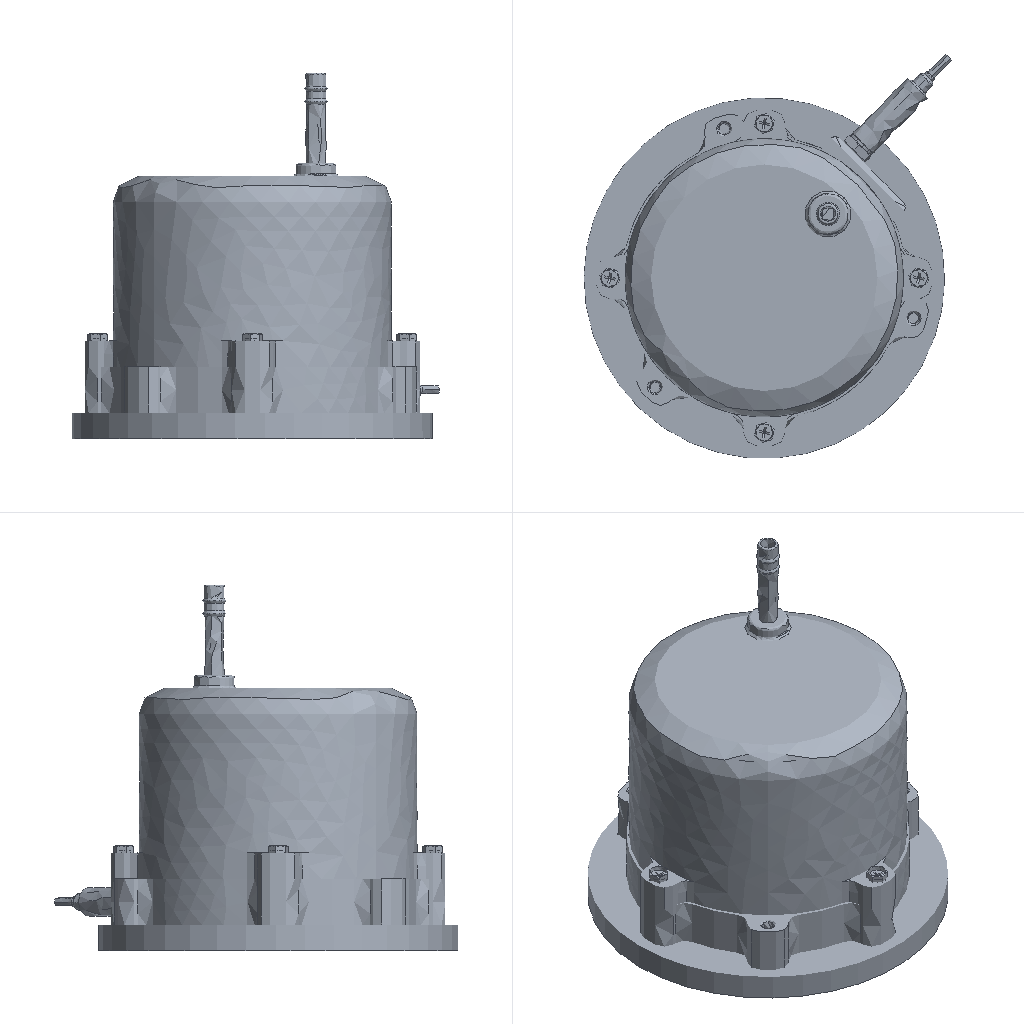Simulation study | ansys workbench
Ansys APDL input file, long lists of numbers shortened:
/batch
/config,noeldb,1     ! force off writing results to database
*get,_wallstrt,active,,time,wall
! ANSYS input file written by Workbench version 2022 R1
! File used for geometry attach:
/title,_________--__ (B5)
! ****** Begin Custom Load Command Snippet ******
/COM, ACT Extensions:
/COM,     LSDYNA, 2021.1
/COM,
! ****** End   Custom Load Command Snippet ******
*DIM,_wb_ProjectScratch_dir,string,248
_wb_ProjectScratch_dir(1) = ''
*DIM,_wb_SolverFiles_dir,string,248
_wb_SolverFiles_dir(1) = ''
*DIM,_wb_userfiles_dir,string,248
_wb_userfiles_dir(1) = ''
/com,--- Data in consistent NMM units. See Solving Units in the help system for more information.
/units,MPA
/nopr
/wb,file,start              !  signify a WB generated input file
/prep7
! Turn off shape checking because checks already performed inside WB mesher.
! See help system for more information.
SHPP,OFF,,NOWARN
/nolist
etcon,set             ! allow ANSYS to choose best KEYOP's for 180x elements, resets any applicable keyopt to MAPDL defaults
/com,*********** Nodes for the whole assembly ***********
nblock,3,,121147
(1i9,3e20.9e3)
        1    -1.317994642E+02     2.267337416E+01     2.460000000E+01
! (110133 more lines like these left out)
-1
/wb,elem,start            !  set before creation of elements
/com,*********** Elements for Body 1 "___|__-__3" ***********
et,1,187
eblock,19,solid,,437
(19i9)
        1        1        1        1        0        0        0        0       10        0     4342    11800    11908    11828    11837    12339    12480    12336    12337
! (873 more lines like these left out)
-1
/com,*********** Elements for Body 2 "__|__1" ***********
et,2,187
eblock,19,solid,,16989
(19i9)
        2        2        2        2        0        0        0        0       10        0    40629    81691    81703    85517    85507    90407    90536    90413    90412
! (33977 more lines like these left out)
-1
/com,*********** Elements for Body 3 "___|__-__1" ***********
et,3,186
keyo,3,2,1          ! set full integration on SOLID186
eblock,19,solid,,126
(19i9)
        3        3        3        3        0        0        0        0       20        0     2518     7295     7301     7355     7349     7392     7391     7382     7383
! (251 more lines like these left out)
-1
/com,*********** Elements for Body 4 "_|__-__3" ***********
et,4,187
eblock,19,solid,,3042
(19i9)
        4        4        4        4        0        0        0        0       10        0    14075    32512    32947    32813    32928    35736    37332    35733    35735
! (6083 more lines like these left out)
-1
/com,*********** Elements for Body 5 "__|__-__1" ***********
et,5,187
eblock,19,solid,,690
(19i9)
        5        5        5        5        0        0        0        0       10        0     9765    23012    23027    23014    23415    23498    23512    23496    23501
! (1379 more lines like these left out)
-1
! (25 more sections like these left out)
/wb,elem,end               !  done creating elements
/com,*********** Send User Defined Coordinate System(s) ***********
csys,0
toffst,273.15,  ! Temperature offset from absolute zero
/com,*********** Set Reference Temperature ***********
tref,22.
/wb,mat,start              !  starting to send materials
/com,*********** Send Materials ***********
Temperature = 'TEMP' ! Temperature
MP,DENS,1,7.85e-09,	! tonne mm^-3
MP,ALPX,1,1.2e-05,	! C^-1
MP,C,1,434000000,	! mm^2 s^-2 C^-1
MP,KXX,1,60.5,	! tonne mm s^-3 C^-1
MP,RSVX,1,0.00017,	! ohm mm
MP,EX,1,200000,	! tonne s^-2 mm^-1
MP,NUXY,1,0.3,
MP,MURX,1,10000,
Temperature = 'TEMP' ! Temperature
MP,DENS,2,7.85e-09,	! tonne mm^-3
MP,ALPX,2,1.2e-05,	! C^-1
MP,C,2,434000000,	! mm^2 s^-2 C^-1
MP,KXX,2,60.5,	! tonne mm s^-3 C^-1
MP,RSVX,2,0.00017,	! ohm mm
MP,EX,2,200000,	! tonne s^-2 mm^-1
MP,NUXY,2,0.3,
MP,MURX,2,10000,
Temperature = 'TEMP' ! Temperature
MP,DENS,3,7.85e-09,	! tonne mm^-3
MP,ALPX,3,1.2e-05,	! C^-1
MP,C,3,434000000,	! mm^2 s^-2 C^-1
MP,KXX,3,60.5,	! tonne mm s^-3 C^-1
MP,RSVX,3,0.00017,	! ohm mm
MP,EX,3,200000,	! tonne s^-2 mm^-1
MP,NUXY,3,0.3,
MP,MURX,3,10000,
Temperature = 'TEMP' ! Temperature
MP,DENS,4,7.85e-09,	! tonne mm^-3
MP,ALPX,4,1.2e-05,	! C^-1
MP,C,4,434000000,	! mm^2 s^-2 C^-1
MP,KXX,4,60.5,	! tonne mm s^-3 C^-1
MP,RSVX,4,0.00017,	! ohm mm
MP,EX,4,200000,	! tonne s^-2 mm^-1
MP,NUXY,4,0.3,
MP,MURX,4,10000,
Temperature = 'TEMP' ! Temperature
MP,DENS,5,7.85e-09,	! tonne mm^-3
MP,ALPX,5,1.2e-05,	! C^-1
MP,C,5,434000000,	! mm^2 s^-2 C^-1
MP,KXX,5,60.5,	! tonne mm s^-3 C^-1
MP,RSVX,5,0.00017,	! ohm mm
MP,EX,5,200000,	! tonne s^-2 mm^-1
MP,NUXY,5,0.3,
MP,MURX,5,10000,
Temperature = 'TEMP' ! Temperature
MP,DENS,6,7.85e-09,	! tonne mm^-3
MP,ALPX,6,1.2e-05,	! C^-1
MP,C,6,434000000,	! mm^2 s^-2 C^-1
MP,KXX,6,60.5,	! tonne mm s^-3 C^-1
MP,RSVX,6,0.00017,	! ohm mm
MP,EX,6,200000,	! tonne s^-2 mm^-1
MP,NUXY,6,0.3,
MP,MURX,6,10000,
Temperature = 'TEMP' ! Temperature
MP,DENS,7,7.85e-09,	! tonne mm^-3
MP,ALPX,7,1.2e-05,	! C^-1
MP,C,7,434000000,	! mm^2 s^-2 C^-1
MP,KXX,7,60.5,	! tonne mm s^-3 C^-1
MP,RSVX,7,0.00017,	! ohm mm
MP,EX,7,200000,	! tonne s^-2 mm^-1
MP,NUXY,7,0.3,
MP,MURX,7,10000,
Temperature = 'TEMP' ! Temperature
MP,DENS,8,7.85e-09,	! tonne mm^-3
MP,ALPX,8,1.2e-05,	! C^-1
MP,C,8,434000000,	! mm^2 s^-2 C^-1
MP,KXX,8,60.5,	! tonne mm s^-3 C^-1
MP,RSVX,8,0.00017,	! ohm mm
MP,EX,8,200000,	! tonne s^-2 mm^-1
MP,NUXY,8,0.3,
MP,MURX,8,10000,
Temperature = 'TEMP' ! Temperature
MP,DENS,9,7.85e-09,	! tonne mm^-3
MP,ALPX,9,1.2e-05,	! C^-1
MP,C,9,434000000,	! mm^2 s^-2 C^-1
MP,KXX,9,60.5,	! tonne mm s^-3 C^-1
MP,RSVX,9,0.00017,	! ohm mm
MP,EX,9,200000,	! tonne s^-2 mm^-1
! (191 more lines like these left out)
/wb,mat,end                !  done sending materials
!************************* Model Summary ********************
!___|__-__3,	结构钢,	matid,	1
!__|__1,	结构钢,	matid,	2
!___|__-__1,	结构钢,	matid,	3
! (29 more lines like these left out)
*get,_xmin,node,,mnloc,x
*get,_ymin,node,,mnloc,y
*get,_zmin,node,,mnloc,z
*get,_xmax,node,,mxloc,x
*get,_ymax,node,,mxloc,y
*get,_zmax,node,,mxloc,z
_ASMDIAG=(_xmax-_xmin)*(_xmax-_xmin)+(_ymax-_ymin)*(_ymax-_ymin)+(_zmax-_zmin)*(_zmax-_zmin)
_ASMDIAG=SQRT(_ASMDIAG)
/wb,contact,start          !  starting to send contact
/com,*********** Create Contact "接触区域" ***********
/com,            Real Constant Set For Above Contact Is 32 & 31
*set,tid,32
*set,cid,31
r,tid
r,cid
et,tid,170
et,cid,174
eblock,10,,,43
(15i9)
   143366       32       32       32        0    11758    11844    11822    11822    12118    12445    11822    12116
! (42 more lines like these left out)
-1
eblock,10,,,43
(15i9)
   143409       31       31       31        0    11758    11844    11822    11822    12118    12445    11822    12116
! (42 more lines like these left out)
-1
eblock,10,,,120
(15i9)
   143452       31       32       31        0    82039    83753    83114    83114    92781    99180    83114    92780
! (119 more lines like these left out)
-1
eblock,10,,,120
(15i9)
   143572       32       31       32        0    82039    83753    83114    83114    92781    99180    83114    92780
! (119 more lines like these left out)
-1
keyo,cid,8,2               ! auto create asymmetric contact (from Program Controlled setting)
keyo,cid,10,0              ! adjust contact stiffness each NR iteration (from Program Controlled setting)
keyo,cid,12,5              ! bonded always
keyo,cid,18,1              ! small sliding turned on by application
keyo,cid,2,0               ! augmented Lagrange (from Program Controlled setting)
keyo,cid,4,0               ! on Gauss point (from Program Controlled setting)
keyo,cid,9,1               ! ignore initial gaps/penetration
keyo,cid,7,0               ! No Prediction
rmod,tid,3,10.      ! FKN
rmod,tid,5,0.       ! ICONT
rmod,tid,6,0.       ! PINB
rmod,tid,10,0.      ! CNOF
rmod,tid,12,0.      ! FKT
rmod,tid,36,116     ! WB DSID
rmod,cid,3,10.      ! FKN
rmod,cid,5,0.       ! ICONT
rmod,cid,6,0.       ! PINB
rmod,cid,10,0.      ! CNOF
rmod,cid,12,0.      ! FKT
rmod,cid,36,116     ! WB DSID
/com,*********** Create Contact "接触区域 3" ***********
/com,            Real Constant Set For Above Contact Is 34 & 33
*set,tid,34
*set,cid,33
r,tid
r,cid
et,tid,170
et,cid,174
eblock,10,,,41
(15i9)
   143692       34       34       34        0    11878    11879    11880    11880    12653    12660    11880    12654
! (40 more lines like these left out)
-1
eblock,10,,,41
(15i9)
   143733       33       33       33        0    11878    11879    11880    11880    12653    12660    11880    12654
! (40 more lines like these left out)
-1
eblock,10,,,64
(15i9)
   143774       33       34       33        0       90       57       14       13      304      185      181      183
! (63 more lines like these left out)
-1
eblock,10,,,64
(15i9)
   143838       34       33       34        0       90       57       14       13      304      185      181      183
! (63 more lines like these left out)
-1
keyo,cid,8,2               ! auto create asymmetric contact (from Program Controlled setting)
keyo,cid,10,0              ! adjust contact stiffness each NR iteration (from Program Controlled setting)
keyo,cid,12,5              ! bonded always
keyo,cid,18,1              ! small sliding turned on by application
keyo,cid,2,0               ! augmented Lagrange (from Program Controlled setting)
keyo,cid,4,0               ! on Gauss point (from Program Controlled setting)
keyo,cid,9,1               ! ignore initial gaps/penetration
keyo,cid,7,0               ! No Prediction
rmod,tid,3,10.      ! FKN
rmod,tid,5,0.       ! ICONT
rmod,tid,6,0.       ! PINB
rmod,tid,10,0.      ! CNOF
rmod,tid,12,0.      ! FKT
rmod,tid,36,122     ! WB DSID
rmod,cid,3,10.      ! FKN
rmod,cid,5,0.       ! ICONT
rmod,cid,6,0.       ! PINB
rmod,cid,10,0.      ! CNOF
rmod,cid,12,0.      ! FKT
rmod,cid,36,122     ! WB DSID
/com,*********** Create Contact "接触区域 4" ***********
/com,            Real Constant Set For Above Contact Is 36 & 35
*set,tid,36
*set,cid,35
r,tid
r,cid
et,tid,170
et,cid,174
eblock,10,,,39
(15i9)
   143902       36       36       36        0    11761    11876    11877    11877    12134    12647    11877    12135
! (38 more lines like these left out)
-1
eblock,10,,,39
(15i9)
   143941       35       35       35        0    11761    11876    11877    11877    12134    12647    11877    12135
! (38 more lines like these left out)
-1
eblock,10,,,64
(15i9)
   143980       35       36       35        0      562      529      486      485      776      657      653      655
! (63 more lines like these left out)
-1
eblock,10,,,64
(15i9)
   144044       36       35       36        0      562      529      486      485      776      657      653      655
! (63 more lines like these left out)
-1
keyo,cid,8,2               ! auto create asymmetric contact (from Program Controlled setting)
keyo,cid,10,0              ! adjust contact stiffness each NR iteration (from Program Controlled setting)
keyo,cid,12,5              ! bonded always
keyo,cid,18,1              ! small sliding turned on by application
keyo,cid,2,0               ! augmented Lagrange (from Program Controlled setting)
keyo,cid,4,0               ! on Gauss point (from Program Controlled setting)
keyo,cid,9,1               ! ignore initial gaps/penetration
keyo,cid,7,0               ! No Prediction
rmod,tid,3,10.      ! FKN
rmod,tid,5,0.       ! ICONT
rmod,tid,6,0.       ! PINB
rmod,tid,10,0.      ! CNOF
rmod,tid,12,0.      ! FKT
rmod,tid,36,125     ! WB DSID
rmod,cid,3,10.      ! FKN
rmod,cid,5,0.       ! ICONT
rmod,cid,6,0.       ! PINB
rmod,cid,10,0.      ! CNOF
rmod,cid,12,0.      ! FKT
rmod,cid,36,125     ! WB DSID
/com,*********** Create Contact "接触区域 5" ***********
/com,            Real Constant Set For Above Contact Is 38 & 37
*set,tid,38
*set,cid,37
r,tid
r,cid
et,tid,170
et,cid,174
eblock,10,,,34
(15i9)
   144108       38       38       38        0    11778    11867    11861    11861    12232    12603    11861    12230
! (33 more lines like these left out)
-1
eblock,10,,,34
(15i9)
   144142       37       37       37        0    11778    11867    11861    11861    12232    12603    11861    12230
! (33 more lines like these left out)
-1
eblock,10,,,483
(15i9)
   144176       37       38       37        0    47491    47545    47546    47546    58831    59057    47546    58832
! (482 more lines like these left out)
-1
eblock,10,,,483
(15i9)
   144659       38       37       38        0    47491    47545    47546    47546    58831    59057    47546    58832
! (482 more lines like these left out)
-1
keyo,cid,8,2               ! auto create asymmetric contact (from Program Controlled setting)
keyo,cid,10,0              ! adjust contact stiffness each NR iteration (from Program Controlled setting)
keyo,cid,12,5              ! bonded always
keyo,cid,18,1              ! small sliding turned on by application
keyo,cid,2,0               ! augmented Lagrange (from Program Controlled setting)
keyo,cid,4,0               ! on Gauss point (from Program Controlled setting)
keyo,cid,9,1               ! ignore initial gaps/penetration
keyo,cid,7,0               ! No Prediction
rmod,tid,3,10.      ! FKN
rmod,tid,5,0.       ! ICONT
rmod,tid,6,0.       ! PINB
rmod,tid,10,0.      ! CNOF
rmod,tid,12,0.      ! FKT
rmod,tid,36,128     ! WB DSID
rmod,cid,3,10.      ! FKN
rmod,cid,5,0.       ! ICONT
rmod,cid,6,0.       ! PINB
rmod,cid,10,0.      ! CNOF
rmod,cid,12,0.      ! FKT
rmod,cid,36,128     ! WB DSID
/com,*********** Create Contact "接触区域 6" ***********
/com,            Real Constant Set For Above Contact Is 40 & 39
*set,tid,40
*set,cid,39
r,tid
r,cid
et,tid,170
et,cid,174
eblock,10,,,35
(15i9)
   145142       40       40       40        0    11778    11867    11861    11861    12232    12603    11861    12230
! (34 more lines like these left out)
-1
eblock,10,,,35
(15i9)
   145177       39       39       39        0    11778    11867    11861    11861    12232    12603    11861    12230
! (34 more lines like these left out)
-1
eblock,10,,,492
(15i9)
   145212       39       40       39        0    64097    65363    64098    64098    68465    68470    64098    68462
! (491 more lines like these left out)
-1
eblock,10,,,492
(15i9)
   145704       40       39       40        0    64097    65363    64098    64098    68465    68470    64098    68462
! (491 more lines like these left out)
-1
keyo,cid,8,2               ! auto create asymmetric contact (from Program Controlled setting)
keyo,cid,10,0              ! adjust contact stiffness each NR iteration (from Program Controlled setting)
keyo,cid,12,5              ! bonded always
keyo,cid,18,1              ! small sliding turned on by application
keyo,cid,2,0               ! augmented Lagrange (from Program Controlled setting)
keyo,cid,4,0               ! on Gauss point (from Program Controlled setting)
keyo,cid,9,1               ! ignore initial gaps/penetration
keyo,cid,7,0               ! No Prediction
rmod,tid,3,10.      ! FKN
rmod,tid,5,0.       ! ICONT
rmod,tid,6,0.       ! PINB
rmod,tid,10,0.      ! CNOF
rmod,tid,12,0.      ! FKT
rmod,tid,36,131     ! WB DSID
rmod,cid,3,10.      ! FKN
rmod,cid,5,0.       ! ICONT
rmod,cid,6,0.       ! PINB
rmod,cid,10,0.      ! CNOF
rmod,cid,12,0.      ! FKT
rmod,cid,36,131     ! WB DSID
! (48 more sections like these left out)
/wb,contact,end            !  done creating contacts
/golist
/wb,load,start             !  starting to send loads
CMBLOCK,_CM332_FIXEDSU,NODE,      333
(8i10)
     17821     17822     17823     17824     17829     17830     17831     17832
! (41 more lines like these left out)
/com,*********** Fixed Supports ***********
CMBLOCK,_FIXEDSU,NODE,      333
(8i10)
     17821     17822     17823     17824     17829     17830     17831     17832
! (41 more lines like these left out)
cmsel,s,_FIXEDSU
d,all,all
nsel,all
/gst,on,on
fini
*get,_numnode,node,0,count
*get,_numelem,elem,0,count
*get, _MAXELEMNUM, elem, 0, NUM, MAX
*get, _MAXNODENUM, node, 0, NUM, MAX
*get, _MAXELEMTYPE, etyp, 0, NUM, MAX
*get, _MAXREALCONST, real, 0, NUM, MAX
/go
/wb,load,end               !  done creating loads
/com,--- Number of total nodes = %_numnode%
/com,--- Number of contact elements = 20844
/com,--- Number of spring elements = 0
/com,--- Number of bearing elements = 0
/com,--- Number of solid elements = 57617
/com,--- Number of condensed parts = 0
/com,--- Number of total elements = %_numelem%
*get,_wallbsol,active,,time,wall
/solu
antype,2                   ! modal analysis
_thickRatio=0.267   ! Ratio of thick parts in the model
modopt,lanb,6
outres,erase
outres,all,none
outres,nsol,all
outres,etmp,all
outres,strs,all
outres,epel,all
outres,eppl,all
outres,rsol,all
nsel,s,d,U
nsel,a,d,ROT
esln
cm,_ConstrainedNodes,elem  ! -- reduced set with only constrained nodes
nsel,all
esel,all
outres,nload,all,_ConstrainedNodes  !-- reduced set with only constrained nodes
mxpand,,,,yes,,no             ! expand requested element results, but not write them to file.mode
dmpopt,esav,no
dmpopt,emat,no
dmpopt,full,no
! *********** WB SOLVE COMMAND ***********
! check interactive state
*get,ANSINTER_,active,,int
*if,ANSINTER_,ne,0,then
/eof
*endif
solve
/com *************** Write FE CONNECTORS *********
CEWRITE,file,ce,,INTE
*get,_nmodalsolproc,active,0,numcpu
fini
save,file,db
/nopr
*get,_numnode,node,0,count
*get,_numelem,elem,0,count
*get, _MAXELEMNUM, elem, 0, NUM, MAX
*get, _MAXNODENUM, node, 0, NUM, MAX,,,INTERNAL
*get, _MAXELEMTYPE, etyp, 0, NUM, MAX
*get, _MAXREALCONST, real, 0, NUM, MAX
/gopr
*get,_wallasol,active,,time,wall
/post1
/nopr
*dim,_direction,CHAR,6,1
_direction(1) = 'X'
_direction(2) = 'Y'
_direction(3) = 'Z'
_direction(4) = 'ROTX'
_direction(5) = 'ROTY'
_direction(6) = 'ROTZ'
*get,_lastLS,active,0,set,LSTP
*get,_beginset,active,0,set,nset,first,_lastLS
*get,_endset,active,0,set,nset,last,_lastLS
_nummodes = 0
*if,_endset,gt,0,then
_nummodes = _endset - _beginset + 1
*endif
*do,i_mode,1,_nummodes
   *do,j_component,1,6
			*get,PFACT_%i_mode%_%j_component%,MODE,%i_mode%,PFACT,,DIREC,_direction(%j_component%)
   *enddo
*enddo
*dim,_tmdirection,CHAR,6,1
_tmdirection(1) = 'X'
_tmdirection(2) = 'Y'
_tmdirection(3) = 'Z'
_tmdirection(4) = 'X'
_tmdirection(5) = 'Y'
_tmdirection(6) = 'Z'
*do,j_component,1,6
    *if,j_component,gt,3,then
        *get,TOTALMASS_%j_component%,ELEM,0,IOR,_tmdirection(%j_component%)
    *else
        *get,TOTALMASS_%j_component%,ELEM,0,MTOT,_tmdirection(%j_component%)
    *endif
*enddo
/gopr
xmlo,ENCODING,ISO-8859-1
xmlo,parm
/xml,parm,xml
fini
/gopr
*get,_walldone,active,,time,wall
_preptime=(_wallbsol-_wallstrt)*3600
_solvtime=(_wallasol-_wallbsol)*3600
_posttime=(_walldone-_wallasol)*3600
_totaltim=(_walldone-_wallstrt)*3600
*get,_dlbratio,active,0,solu,dlbr
*get,_combtime,active,0,solu,comb
*get,_ssmode,active,0,solu,ssmm
*get,_ndofs,active,0,solu,ndof
/com,--- Total number of nodes = %_numnode%
/com,--- Total number of elements = %_numelem%
/com,--- Element load balance ratio = %_dlbratio%
/com,--- Time to combine distributed files = %_combtime%
/com,--- Sparse memory mode = %_ssmode%
/com,--- Number of DOF = %_ndofs%
/wb,file,end               ! done with WB generated input